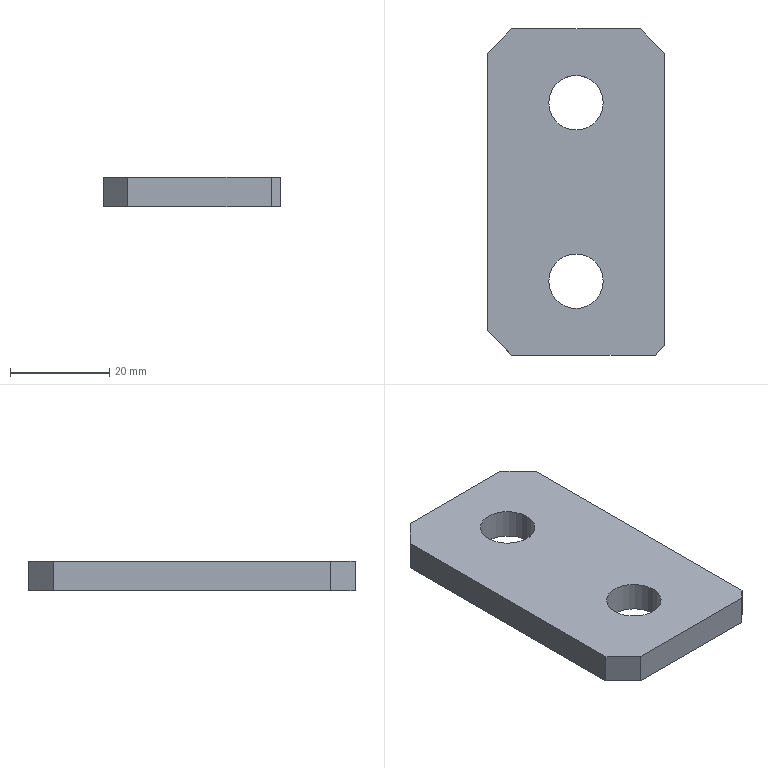Part | STEP file | 1_id134_x_t | 1 solid | 12 faces | box 35.8 x 65.8 x 6 mm | volume 12762 mm3 | plane 10 | cylinder 2 | commonest cylinder face diameters 11 x2
STEP:
#1=CARTESIAN_POINT('',(0.,0.,0.));
#2=DIRECTION('',(0.,0.,1.));
#3=DIRECTION('',(1.,0.,0.));
#4=AXIS2_PLACEMENT_3D('',#1,#2,#3);
#5=CARTESIAN_POINT('',(51.316,210.4,84.11));
#6=VERTEX_POINT('',#5);
#7=CARTESIAN_POINT('',(46.375,205.459,84.11));
#8=VERTEX_POINT('',#7);
#9=CARTESIAN_POINT('',(32.346,191.429,84.11));
#10=DIRECTION('',(-0.7071,-0.7071,0.));
#11=VECTOR('',#10,1.);
#12=LINE('',#9,#11);
#13=CARTESIAN_POINT('',(51.346,210.429,90.11));
#14=DIRECTION('',(0.7071,-0.7071,0.));
#15=DIRECTION('',(0.7071,0.7071,0.));
#16=AXIS2_PLACEMENT_3D('',#13,#14,#15);
#17=PLANE('',#16);
#18=CARTESIAN_POINT('',(-26.87,-6.));
#19=DIRECTION('',(-1.,0.));
#20=VECTOR('',#19,1.);
#21=LINE('',#18,#20);
#22=(GEOMETRIC_REPRESENTATION_CONTEXT(2)PARAMETRIC_REPRESENTATION_CONTEXT()REPRESENTATION_CONTEXT('',''));
#23=DEFINITIONAL_REPRESENTATION('',(#21),#22);
#24=PCURVE('',#17,#23);
#25=CARTESIAN_POINT('',(64.275,159.5,84.11));
#26=DIRECTION('',(0.,0.,-1.));
#27=DIRECTION('',(-1.,0.,0.));
#28=AXIS2_PLACEMENT_3D('',#25,#26,#27);
#29=PLANE('',#28);
#30=CARTESIAN_POINT('',(31.929,31.929));
#31=DIRECTION('',(0.7071,-0.7071));
#32=VECTOR('',#31,1.);
#33=LINE('',#30,#32);
#34=(GEOMETRIC_REPRESENTATION_CONTEXT(2)PARAMETRIC_REPRESENTATION_CONTEXT()REPRESENTATION_CONTEXT('',''));
#35=DEFINITIONAL_REPRESENTATION('',(#33),#34);
#36=PCURVE('',#29,#35);
#37=SURFACE_CURVE('',#12,(#24,#36),.PCURVE_S1.);
#38=EDGE_CURVE('',#6,#8,#37,.T.);
#39=ORIENTED_EDGE('',*,*,#38,.T.);
#40=CARTESIAN_POINT('',(46.375,205.459,90.11));
#41=VERTEX_POINT('',#40);
#42=CARTESIAN_POINT('',(46.375,205.459,90.11));
#43=DIRECTION('',(0.,0.,-1.));
#44=VECTOR('',#43,1.);
#45=LINE('',#42,#44);
#46=CARTESIAN_POINT('',(-7.03,0.));
#47=DIRECTION('',(0.,-1.));
#48=VECTOR('',#47,1.);
#49=LINE('',#46,#48);
#50=(GEOMETRIC_REPRESENTATION_CONTEXT(2)PARAMETRIC_REPRESENTATION_CONTEXT()REPRESENTATION_CONTEXT('',''));
#51=DEFINITIONAL_REPRESENTATION('',(#49),#50);
#52=PCURVE('',#17,#51);
#53=CARTESIAN_POINT('',(46.375,205.5,90.11));
#54=DIRECTION('',(1.,0.,0.));
#55=DIRECTION('',(0.,0.,-1.));
#56=AXIS2_PLACEMENT_3D('',#53,#54,#55);
#57=PLANE('',#56);
#58=CARTESIAN_POINT('',(0.,-0.04142));
#59=DIRECTION('',(1.,0.));
#60=VECTOR('',#59,1.);
#61=LINE('',#58,#60);
#62=(GEOMETRIC_REPRESENTATION_CONTEXT(2)PARAMETRIC_REPRESENTATION_CONTEXT()REPRESENTATION_CONTEXT('',''));
#63=DEFINITIONAL_REPRESENTATION('',(#61),#62);
#64=PCURVE('',#57,#63);
#65=SURFACE_CURVE('',#45,(#52,#64),.PCURVE_S1.);
#66=EDGE_CURVE('',#41,#8,#65,.T.);
#67=ORIENTED_EDGE('',*,*,#66,.F.);
#68=CARTESIAN_POINT('',(51.316,210.4,90.11));
#69=VERTEX_POINT('',#68);
#70=CARTESIAN_POINT('',(32.346,191.429,90.11));
#71=DIRECTION('',(-0.7071,-0.7071,0.));
#72=VECTOR('',#71,1.);
#73=LINE('',#70,#72);
#74=CARTESIAN_POINT('',(-26.87,0.));
#75=DIRECTION('',(-1.,0.));
#76=VECTOR('',#75,1.);
#77=LINE('',#74,#76);
#78=(GEOMETRIC_REPRESENTATION_CONTEXT(2)PARAMETRIC_REPRESENTATION_CONTEXT()REPRESENTATION_CONTEXT('',''));
#79=DEFINITIONAL_REPRESENTATION('',(#77),#78);
#80=PCURVE('',#17,#79);
#81=CARTESIAN_POINT('',(64.275,159.5,90.11));
#82=DIRECTION('',(0.,0.,-1.));
#83=DIRECTION('',(-1.,0.,0.));
#84=AXIS2_PLACEMENT_3D('',#81,#82,#83);
#85=PLANE('',#84);
#86=CARTESIAN_POINT('',(31.929,31.929));
#87=DIRECTION('',(0.7071,-0.7071));
#88=VECTOR('',#87,1.);
#89=LINE('',#86,#88);
#90=(GEOMETRIC_REPRESENTATION_CONTEXT(2)PARAMETRIC_REPRESENTATION_CONTEXT()REPRESENTATION_CONTEXT('',''));
#91=DEFINITIONAL_REPRESENTATION('',(#89),#90);
#92=PCURVE('',#85,#91);
#93=SURFACE_CURVE('',#73,(#80,#92),.PCURVE_S1.);
#94=EDGE_CURVE('',#69,#41,#93,.T.);
#95=ORIENTED_EDGE('',*,*,#94,.F.);
#96=CARTESIAN_POINT('',(51.316,210.4,90.11));
#97=DIRECTION('',(0.,0.,-1.));
#98=VECTOR('',#97,1.);
#99=LINE('',#96,#98);
#100=CARTESIAN_POINT('',(-0.04142,0.));
#101=DIRECTION('',(0.,-1.));
#102=VECTOR('',#101,1.);
#103=LINE('',#100,#102);
#104=(GEOMETRIC_REPRESENTATION_CONTEXT(2)PARAMETRIC_REPRESENTATION_CONTEXT()REPRESENTATION_CONTEXT('',''));
#105=DEFINITIONAL_REPRESENTATION('',(#103),#104);
#106=PCURVE('',#17,#105);
#107=CARTESIAN_POINT('',(77.275,210.4,90.11));
#108=DIRECTION('',(0.,-1.,0.));
#109=DIRECTION('',(0.,0.,-1.));
#110=AXIS2_PLACEMENT_3D('',#107,#108,#109);
#111=PLANE('',#110);
#112=CARTESIAN_POINT('',(0.,-25.959));
#113=DIRECTION('',(1.,0.));
#114=VECTOR('',#113,1.);
#115=LINE('',#112,#114);
#116=(GEOMETRIC_REPRESENTATION_CONTEXT(2)PARAMETRIC_REPRESENTATION_CONTEXT()REPRESENTATION_CONTEXT('',''));
#117=DEFINITIONAL_REPRESENTATION('',(#115),#116);
#118=PCURVE('',#111,#117);
#119=SURFACE_CURVE('',#99,(#106,#118),.PCURVE_S1.);
#120=EDGE_CURVE('',#69,#6,#119,.T.);
#121=ORIENTED_EDGE('',*,*,#120,.T.);
#122=EDGE_LOOP('',(#39,#67,#95,#121));
#123=FACE_BOUND('',#122,.T.);
#124=ADVANCED_FACE('',(#123),#17,.F.);
#125=CARTESIAN_POINT('',(46.375,149.541,84.11));
#126=VERTEX_POINT('',#125);
#127=CARTESIAN_POINT('',(46.375,159.5,84.11));
#128=DIRECTION('',(0.,-1.,0.));
#129=VECTOR('',#128,1.);
#130=LINE('',#127,#129);
#131=CARTESIAN_POINT('',(6.,-46.));
#132=DIRECTION('',(0.,-1.));
#133=VECTOR('',#132,1.);
#134=LINE('',#131,#133);
#135=(GEOMETRIC_REPRESENTATION_CONTEXT(2)PARAMETRIC_REPRESENTATION_CONTEXT()REPRESENTATION_CONTEXT('',''));
#136=DEFINITIONAL_REPRESENTATION('',(#134),#135);
#137=PCURVE('',#57,#136);
#138=CARTESIAN_POINT('',(17.9,0.));
#139=DIRECTION('',(0.,-1.));
#140=VECTOR('',#139,1.);
#141=LINE('',#138,#140);
#142=(GEOMETRIC_REPRESENTATION_CONTEXT(2)PARAMETRIC_REPRESENTATION_CONTEXT()REPRESENTATION_CONTEXT('',''));
#143=DEFINITIONAL_REPRESENTATION('',(#141),#142);
#144=PCURVE('',#29,#143);
#145=SURFACE_CURVE('',#130,(#137,#144),.PCURVE_S1.);
#146=EDGE_CURVE('',#8,#126,#145,.T.);
#147=ORIENTED_EDGE('',*,*,#146,.T.);
#148=CARTESIAN_POINT('',(46.375,149.541,90.11));
#149=VERTEX_POINT('',#148);
#150=CARTESIAN_POINT('',(46.375,149.541,90.11));
#151=DIRECTION('',(0.,0.,-1.));
#152=VECTOR('',#151,1.);
#153=LINE('',#150,#152);
#154=CARTESIAN_POINT('',(0.,-55.959));
#155=DIRECTION('',(1.,0.));
#156=VECTOR('',#155,1.);
#157=LINE('',#154,#156);
#158=(GEOMETRIC_REPRESENTATION_CONTEXT(2)PARAMETRIC_REPRESENTATION_CONTEXT()REPRESENTATION_CONTEXT('',''));
#159=DEFINITIONAL_REPRESENTATION('',(#157),#158);
#160=PCURVE('',#57,#159);
#161=CARTESIAN_POINT('',(46.346,149.571,90.11));
#162=DIRECTION('',(0.7071,0.7071,0.));
#163=DIRECTION('',(-0.7071,0.7071,0.));
#164=AXIS2_PLACEMENT_3D('',#161,#162,#163);
#165=PLANE('',#164);
#166=CARTESIAN_POINT('',(-0.04142,0.));
#167=DIRECTION('',(0.,-1.));
#168=VECTOR('',#167,1.);
#169=LINE('',#166,#168);
#170=(GEOMETRIC_REPRESENTATION_CONTEXT(2)PARAMETRIC_REPRESENTATION_CONTEXT()REPRESENTATION_CONTEXT('',''));
#171=DEFINITIONAL_REPRESENTATION('',(#169),#170);
#172=PCURVE('',#165,#171);
#173=SURFACE_CURVE('',#153,(#160,#172),.PCURVE_S1.);
#174=EDGE_CURVE('',#149,#126,#173,.T.);
#175=ORIENTED_EDGE('',*,*,#174,.F.);
#176=CARTESIAN_POINT('',(46.375,159.5,90.11));
#177=DIRECTION('',(0.,-1.,0.));
#178=VECTOR('',#177,1.);
#179=LINE('',#176,#178);
#180=CARTESIAN_POINT('',(0.,-46.));
#181=DIRECTION('',(0.,-1.));
#182=VECTOR('',#181,1.);
#183=LINE('',#180,#182);
#184=(GEOMETRIC_REPRESENTATION_CONTEXT(2)PARAMETRIC_REPRESENTATION_CONTEXT()REPRESENTATION_CONTEXT('',''));
#185=DEFINITIONAL_REPRESENTATION('',(#183),#184);
#186=PCURVE('',#57,#185);
#187=CARTESIAN_POINT('',(17.9,0.));
#188=DIRECTION('',(0.,-1.));
#189=VECTOR('',#188,1.);
#190=LINE('',#187,#189);
#191=(GEOMETRIC_REPRESENTATION_CONTEXT(2)PARAMETRIC_REPRESENTATION_CONTEXT()REPRESENTATION_CONTEXT('',''));
#192=DEFINITIONAL_REPRESENTATION('',(#190),#191);
#193=PCURVE('',#85,#192);
#194=SURFACE_CURVE('',#179,(#186,#193),.PCURVE_S1.);
#195=EDGE_CURVE('',#41,#149,#194,.T.);
#196=ORIENTED_EDGE('',*,*,#195,.F.);
#197=ORIENTED_EDGE('',*,*,#66,.T.);
#198=EDGE_LOOP('',(#147,#175,#196,#197));
#199=FACE_BOUND('',#198,.T.);
#200=ADVANCED_FACE('',(#199),#57,.F.);
#201=CARTESIAN_POINT('',(51.316,144.6,84.11));
#202=VERTEX_POINT('',#201);
#203=CARTESIAN_POINT('',(50.346,145.571,84.11));
#204=DIRECTION('',(0.7071,-0.7071,0.));
#205=VECTOR('',#204,1.);
#206=LINE('',#203,#205);
#207=CARTESIAN_POINT('',(-5.657,-6.));
#208=DIRECTION('',(-1.,0.));
#209=VECTOR('',#208,1.);
#210=LINE('',#207,#209);
#211=(GEOMETRIC_REPRESENTATION_CONTEXT(2)PARAMETRIC_REPRESENTATION_CONTEXT()REPRESENTATION_CONTEXT('',''));
#212=DEFINITIONAL_REPRESENTATION('',(#210),#211);
#213=PCURVE('',#165,#212);
#214=CARTESIAN_POINT('',(13.929,-13.929));
#215=DIRECTION('',(-0.7071,-0.7071));
#216=VECTOR('',#215,1.);
#217=LINE('',#214,#216);
#218=(GEOMETRIC_REPRESENTATION_CONTEXT(2)PARAMETRIC_REPRESENTATION_CONTEXT()REPRESENTATION_CONTEXT('',''));
#219=DEFINITIONAL_REPRESENTATION('',(#217),#218);
#220=PCURVE('',#29,#219);
#221=SURFACE_CURVE('',#206,(#213,#220),.PCURVE_S1.);
#222=EDGE_CURVE('',#126,#202,#221,.T.);
#223=ORIENTED_EDGE('',*,*,#222,.T.);
#224=CARTESIAN_POINT('',(51.316,144.6,90.11));
#225=VERTEX_POINT('',#224);
#226=CARTESIAN_POINT('',(51.316,144.6,90.11));
#227=DIRECTION('',(0.,0.,-1.));
#228=VECTOR('',#227,1.);
#229=LINE('',#226,#228);
#230=CARTESIAN_POINT('',(-7.03,0.));
#231=DIRECTION('',(0.,-1.));
#232=VECTOR('',#231,1.);
#233=LINE('',#230,#232);
#234=(GEOMETRIC_REPRESENTATION_CONTEXT(2)PARAMETRIC_REPRESENTATION_CONTEXT()REPRESENTATION_CONTEXT('',''));
#235=DEFINITIONAL_REPRESENTATION('',(#233),#234);
#236=PCURVE('',#165,#235);
#237=CARTESIAN_POINT('',(51.275,144.6,90.11));
#238=DIRECTION('',(0.,1.,0.));
#239=DIRECTION('',(0.,0.,1.));
#240=AXIS2_PLACEMENT_3D('',#237,#238,#239);
#241=PLANE('',#240);
#242=CARTESIAN_POINT('',(0.,0.04142));
#243=DIRECTION('',(-1.,0.));
#244=VECTOR('',#243,1.);
#245=LINE('',#242,#244);
#246=(GEOMETRIC_REPRESENTATION_CONTEXT(2)PARAMETRIC_REPRESENTATION_CONTEXT()REPRESENTATION_CONTEXT('',''));
#247=DEFINITIONAL_REPRESENTATION('',(#245),#246);
#248=PCURVE('',#241,#247);
#249=SURFACE_CURVE('',#229,(#236,#248),.PCURVE_S1.);
#250=EDGE_CURVE('',#225,#202,#249,.T.);
#251=ORIENTED_EDGE('',*,*,#250,.F.);
#252=CARTESIAN_POINT('',(50.346,145.571,90.11));
#253=DIRECTION('',(0.7071,-0.7071,0.));
#254=VECTOR('',#253,1.);
#255=LINE('',#252,#254);
#256=CARTESIAN_POINT('',(-5.657,0.));
#257=DIRECTION('',(-1.,0.));
#258=VECTOR('',#257,1.);
#259=LINE('',#256,#258);
#260=(GEOMETRIC_REPRESENTATION_CONTEXT(2)PARAMETRIC_REPRESENTATION_CONTEXT()REPRESENTATION_CONTEXT('',''));
#261=DEFINITIONAL_REPRESENTATION('',(#259),#260);
#262=PCURVE('',#165,#261);
#263=CARTESIAN_POINT('',(13.929,-13.929));
#264=DIRECTION('',(-0.7071,-0.7071));
#265=VECTOR('',#264,1.);
#266=LINE('',#263,#265);
#267=(GEOMETRIC_REPRESENTATION_CONTEXT(2)PARAMETRIC_REPRESENTATION_CONTEXT()REPRESENTATION_CONTEXT('',''));
#268=DEFINITIONAL_REPRESENTATION('',(#266),#267);
#269=PCURVE('',#85,#268);
#270=SURFACE_CURVE('',#255,(#262,#269),.PCURVE_S1.);
#271=EDGE_CURVE('',#149,#225,#270,.T.);
#272=ORIENTED_EDGE('',*,*,#271,.F.);
#273=ORIENTED_EDGE('',*,*,#174,.T.);
#274=EDGE_LOOP('',(#223,#251,#272,#273));
#275=FACE_BOUND('',#274,.T.);
#276=ADVANCED_FACE('',(#275),#165,.F.);
#277=CARTESIAN_POINT('',(58.775,195.5,84.11));
#278=VERTEX_POINT('',#277);
#279=CARTESIAN_POINT('',(64.275,195.5,84.11));
#280=DIRECTION('',(0.,0.,-1.));
#281=DIRECTION('',(-1.,0.,0.));
#282=AXIS2_PLACEMENT_3D('',#279,#280,#281);
#283=CIRCLE('',#282,5.5);
#284=CARTESIAN_POINT('',(64.275,195.5,90.11));
#285=DIRECTION('',(0.,0.,-1.));
#286=DIRECTION('',(-1.,0.,0.));
#287=AXIS2_PLACEMENT_3D('',#284,#285,#286);
#288=CYLINDRICAL_SURFACE('',#287,5.5);
#289=CARTESIAN_POINT('',(0.,6.));
#290=DIRECTION('',(1.,0.));
#291=VECTOR('',#290,1.);
#292=LINE('',#289,#291);
#293=(GEOMETRIC_REPRESENTATION_CONTEXT(2)PARAMETRIC_REPRESENTATION_CONTEXT()REPRESENTATION_CONTEXT('',''));
#294=DEFINITIONAL_REPRESENTATION('',(#292),#293);
#295=PCURVE('',#288,#294);
#296=CARTESIAN_POINT('',(0.,36.));
#297=DIRECTION('',(1.,0.));
#298=AXIS2_PLACEMENT_2D('',#296,#297);
#299=CIRCLE('',#298,5.5);
#300=(GEOMETRIC_REPRESENTATION_CONTEXT(2)PARAMETRIC_REPRESENTATION_CONTEXT()REPRESENTATION_CONTEXT('',''));
#301=DEFINITIONAL_REPRESENTATION('',(#299),#300);
#302=PCURVE('',#29,#301);
#303=SURFACE_CURVE('',#283,(#295,#302),.PCURVE_S1.);
#304=EDGE_CURVE('',#278,#278,#303,.T.);
#305=ORIENTED_EDGE('',*,*,#304,.F.);
#306=CARTESIAN_POINT('',(58.775,195.5,90.11));
#307=VERTEX_POINT('',#306);
#308=CARTESIAN_POINT('',(58.775,195.5,90.11));
#309=CARTESIAN_POINT('',(58.775,195.5,84.11));
#310=B_SPLINE_CURVE_WITH_KNOTS('',1,(#308,#309),.UNSPECIFIED.,.F.,.F.,(2,2),(0.,6.),.PIECEWISE_BEZIER_KNOTS.);
#311=CARTESIAN_POINT('',(0.,0.));
#312=DIRECTION('',(0.,1.));
#313=VECTOR('',#312,1.);
#314=LINE('',#311,#313);
#315=(GEOMETRIC_REPRESENTATION_CONTEXT(2)PARAMETRIC_REPRESENTATION_CONTEXT()REPRESENTATION_CONTEXT('',''));
#316=DEFINITIONAL_REPRESENTATION('',(#314),#315);
#317=PCURVE('',#288,#316);
#318=CARTESIAN_POINT('',(6.283,0.));
#319=DIRECTION('',(0.,1.));
#320=VECTOR('',#319,1.);
#321=LINE('',#318,#320);
#322=(GEOMETRIC_REPRESENTATION_CONTEXT(2)PARAMETRIC_REPRESENTATION_CONTEXT()REPRESENTATION_CONTEXT('',''));
#323=DEFINITIONAL_REPRESENTATION('',(#321),#322);
#324=PCURVE('',#288,#323);
#325=SEAM_CURVE('',#310,(#317,#324),.PCURVE_S1.);
#326=EDGE_CURVE('',#307,#278,#325,.T.);
#327=ORIENTED_EDGE('',*,*,#326,.F.);
#328=CARTESIAN_POINT('',(64.275,195.5,90.11));
#329=DIRECTION('',(0.,0.,-1.));
#330=DIRECTION('',(-1.,0.,0.));
#331=AXIS2_PLACEMENT_3D('',#328,#329,#330);
#332=CIRCLE('',#331,5.5);
#333=CARTESIAN_POINT('',(0.,0.));
#334=DIRECTION('',(1.,0.));
#335=VECTOR('',#334,1.);
#336=LINE('',#333,#335);
#337=(GEOMETRIC_REPRESENTATION_CONTEXT(2)PARAMETRIC_REPRESENTATION_CONTEXT()REPRESENTATION_CONTEXT('',''));
#338=DEFINITIONAL_REPRESENTATION('',(#336),#337);
#339=PCURVE('',#288,#338);
#340=CARTESIAN_POINT('',(0.,36.));
#341=DIRECTION('',(1.,0.));
#342=AXIS2_PLACEMENT_2D('',#340,#341);
#343=CIRCLE('',#342,5.5);
#344=(GEOMETRIC_REPRESENTATION_CONTEXT(2)PARAMETRIC_REPRESENTATION_CONTEXT()REPRESENTATION_CONTEXT('',''));
#345=DEFINITIONAL_REPRESENTATION('',(#343),#344);
#346=PCURVE('',#85,#345);
#347=SURFACE_CURVE('',#332,(#339,#346),.PCURVE_S1.);
#348=EDGE_CURVE('',#307,#307,#347,.T.);
#349=ORIENTED_EDGE('',*,*,#348,.T.);
#350=ORIENTED_EDGE('',*,*,#326,.T.);
#351=EDGE_LOOP('',(#305,#327,#349,#350));
#352=FACE_BOUND('',#351,.F.);
#353=ADVANCED_FACE('',(#352),#288,.F.);
#354=CARTESIAN_POINT('',(58.775,159.5,84.11));
#355=VERTEX_POINT('',#354);
#356=CARTESIAN_POINT('',(64.275,159.5,84.11));
#357=DIRECTION('',(0.,0.,-1.));
#358=DIRECTION('',(-1.,0.,0.));
#359=AXIS2_PLACEMENT_3D('',#356,#357,#358);
#360=CIRCLE('',#359,5.5);
#361=CARTESIAN_POINT('',(64.275,159.5,90.11));
#362=DIRECTION('',(0.,0.,-1.));
#363=DIRECTION('',(-1.,0.,0.));
#364=AXIS2_PLACEMENT_3D('',#361,#362,#363);
#365=CYLINDRICAL_SURFACE('',#364,5.5);
#366=CARTESIAN_POINT('',(0.,6.));
#367=DIRECTION('',(1.,0.));
#368=VECTOR('',#367,1.);
#369=LINE('',#366,#368);
#370=(GEOMETRIC_REPRESENTATION_CONTEXT(2)PARAMETRIC_REPRESENTATION_CONTEXT()REPRESENTATION_CONTEXT('',''));
#371=DEFINITIONAL_REPRESENTATION('',(#369),#370);
#372=PCURVE('',#365,#371);
#373=CARTESIAN_POINT('',(0.,0.));
#374=DIRECTION('',(1.,0.));
#375=AXIS2_PLACEMENT_2D('',#373,#374);
#376=CIRCLE('',#375,5.5);
#377=(GEOMETRIC_REPRESENTATION_CONTEXT(2)PARAMETRIC_REPRESENTATION_CONTEXT()REPRESENTATION_CONTEXT('',''));
#378=DEFINITIONAL_REPRESENTATION('',(#376),#377);
#379=PCURVE('',#29,#378);
#380=SURFACE_CURVE('',#360,(#372,#379),.PCURVE_S1.);
#381=EDGE_CURVE('',#355,#355,#380,.T.);
#382=ORIENTED_EDGE('',*,*,#381,.F.);
#383=CARTESIAN_POINT('',(58.775,159.5,90.11));
#384=VERTEX_POINT('',#383);
#385=CARTESIAN_POINT('',(58.775,159.5,90.11));
#386=CARTESIAN_POINT('',(58.775,159.5,84.11));
#387=B_SPLINE_CURVE_WITH_KNOTS('',1,(#385,#386),.UNSPECIFIED.,.F.,.F.,(2,2),(0.,6.),.PIECEWISE_BEZIER_KNOTS.);
#388=CARTESIAN_POINT('',(0.,0.));
#389=DIRECTION('',(0.,1.));
#390=VECTOR('',#389,1.);
#391=LINE('',#388,#390);
#392=(GEOMETRIC_REPRESENTATION_CONTEXT(2)PARAMETRIC_REPRESENTATION_CONTEXT()REPRESENTATION_CONTEXT('',''));
#393=DEFINITIONAL_REPRESENTATION('',(#391),#392);
#394=PCURVE('',#365,#393);
#395=CARTESIAN_POINT('',(6.283,0.));
#396=DIRECTION('',(0.,1.));
#397=VECTOR('',#396,1.);
#398=LINE('',#395,#397);
#399=(GEOMETRIC_REPRESENTATION_CONTEXT(2)PARAMETRIC_REPRESENTATION_CONTEXT()REPRESENTATION_CONTEXT('',''));
#400=DEFINITIONAL_REPRESENTATION('',(#398),#399);
#401=PCURVE('',#365,#400);
#402=SEAM_CURVE('',#387,(#394,#401),.PCURVE_S1.);
#403=EDGE_CURVE('',#384,#355,#402,.T.);
#404=ORIENTED_EDGE('',*,*,#403,.F.);
#405=CARTESIAN_POINT('',(64.275,159.5,90.11));
#406=DIRECTION('',(0.,0.,-1.));
#407=DIRECTION('',(-1.,0.,0.));
#408=AXIS2_PLACEMENT_3D('',#405,#406,#407);
#409=CIRCLE('',#408,5.5);
#410=CARTESIAN_POINT('',(0.,0.));
#411=DIRECTION('',(1.,0.));
#412=VECTOR('',#411,1.);
#413=LINE('',#410,#412);
#414=(GEOMETRIC_REPRESENTATION_CONTEXT(2)PARAMETRIC_REPRESENTATION_CONTEXT()REPRESENTATION_CONTEXT('',''));
#415=DEFINITIONAL_REPRESENTATION('',(#413),#414);
#416=PCURVE('',#365,#415);
#417=CARTESIAN_POINT('',(0.,0.));
#418=DIRECTION('',(1.,0.));
#419=AXIS2_PLACEMENT_2D('',#417,#418);
#420=CIRCLE('',#419,5.5);
#421=(GEOMETRIC_REPRESENTATION_CONTEXT(2)PARAMETRIC_REPRESENTATION_CONTEXT()REPRESENTATION_CONTEXT('',''));
#422=DEFINITIONAL_REPRESENTATION('',(#420),#421);
#423=PCURVE('',#85,#422);
#424=SURFACE_CURVE('',#409,(#416,#423),.PCURVE_S1.);
#425=EDGE_CURVE('',#384,#384,#424,.T.);
#426=ORIENTED_EDGE('',*,*,#425,.T.);
#427=ORIENTED_EDGE('',*,*,#403,.T.);
#428=EDGE_LOOP('',(#382,#404,#426,#427));
#429=FACE_BOUND('',#428,.F.);
#430=ADVANCED_FACE('',(#429),#365,.F.);
#431=ORIENTED_EDGE('',*,*,#425,.T.);
#432=EDGE_LOOP('',(#431));
#433=FACE_BOUND('',#432,.T.);
#434=ORIENTED_EDGE('',*,*,#348,.T.);
#435=EDGE_LOOP('',(#434));
#436=FACE_BOUND('',#435,.T.);
#437=CARTESIAN_POINT('',(82.175,146.541,90.11));
#438=VERTEX_POINT('',#437);
#439=CARTESIAN_POINT('',(80.234,144.6,90.11));
#440=VERTEX_POINT('',#439);
#441=CARTESIAN_POINT('',(79.704,144.071,90.11));
#442=DIRECTION('',(-0.7071,-0.7071,0.));
#443=VECTOR('',#442,1.);
#444=LINE('',#441,#443);
#445=CARTESIAN_POINT('',(-15.429,-15.429));
#446=DIRECTION('',(0.7071,-0.7071));
#447=VECTOR('',#446,1.);
#448=LINE('',#445,#447);
#449=(GEOMETRIC_REPRESENTATION_CONTEXT(2)PARAMETRIC_REPRESENTATION_CONTEXT()REPRESENTATION_CONTEXT('',''));
#450=DEFINITIONAL_REPRESENTATION('',(#448),#449);
#451=PCURVE('',#85,#450);
#452=CARTESIAN_POINT('',(80.234,144.6,-90.11));
#453=DIRECTION('',(0.7071,-0.7071,0.));
#454=DIRECTION('',(0.7071,0.7071,0.));
#455=AXIS2_PLACEMENT_3D('',#452,#453,#454);
#456=PLANE('',#455);
#457=CARTESIAN_POINT('',(-0.7485,180.22));
#458=DIRECTION('',(-1.,0.));
#459=VECTOR('',#458,1.);
#460=LINE('',#457,#459);
#461=(GEOMETRIC_REPRESENTATION_CONTEXT(2)PARAMETRIC_REPRESENTATION_CONTEXT()REPRESENTATION_CONTEXT('',''));
#462=DEFINITIONAL_REPRESENTATION('',(#460),#461);
#463=PCURVE('',#456,#462);
#464=SURFACE_CURVE('',#444,(#451,#463),.PCURVE_S1.);
#465=EDGE_CURVE('',#438,#440,#464,.T.);
#466=ORIENTED_EDGE('',*,*,#465,.F.);
#467=CARTESIAN_POINT('',(82.175,205.459,90.11));
#468=VERTEX_POINT('',#467);
#469=CARTESIAN_POINT('',(82.175,159.5,90.11));
#470=DIRECTION('',(0.,1.,0.));
#471=VECTOR('',#470,1.);
#472=LINE('',#469,#471);
#473=CARTESIAN_POINT('',(-17.9,0.));
#474=DIRECTION('',(0.,1.));
#475=VECTOR('',#474,1.);
#476=LINE('',#473,#475);
#477=(GEOMETRIC_REPRESENTATION_CONTEXT(2)PARAMETRIC_REPRESENTATION_CONTEXT()REPRESENTATION_CONTEXT('',''));
#478=DEFINITIONAL_REPRESENTATION('',(#476),#477);
#479=PCURVE('',#85,#478);
#480=CARTESIAN_POINT('',(82.175,149.5,90.11));
#481=DIRECTION('',(-1.,0.,0.));
#482=DIRECTION('',(0.,0.,1.));
#483=AXIS2_PLACEMENT_3D('',#480,#481,#482);
#484=PLANE('',#483);
#485=CARTESIAN_POINT('',(0.,10.));
#486=DIRECTION('',(0.,1.));
#487=VECTOR('',#486,1.);
#488=LINE('',#485,#487);
#489=(GEOMETRIC_REPRESENTATION_CONTEXT(2)PARAMETRIC_REPRESENTATION_CONTEXT()REPRESENTATION_CONTEXT('',''));
#490=DEFINITIONAL_REPRESENTATION('',(#488),#489);
#491=PCURVE('',#484,#490);
#492=SURFACE_CURVE('',#472,(#479,#491),.PCURVE_S1.);
#493=EDGE_CURVE('',#438,#468,#492,.T.);
#494=ORIENTED_EDGE('',*,*,#493,.T.);
#495=CARTESIAN_POINT('',(77.234,210.4,90.11));
#496=VERTEX_POINT('',#495);
#497=CARTESIAN_POINT('',(96.204,191.429,90.11));
#498=DIRECTION('',(0.7071,-0.7071,0.));
#499=VECTOR('',#498,1.);
#500=LINE('',#497,#499);
#501=CARTESIAN_POINT('',(-31.929,31.929));
#502=DIRECTION('',(-0.7071,-0.7071));
#503=VECTOR('',#502,1.);
#504=LINE('',#501,#503);
#505=(GEOMETRIC_REPRESENTATION_CONTEXT(2)PARAMETRIC_REPRESENTATION_CONTEXT()REPRESENTATION_CONTEXT('',''));
#506=DEFINITIONAL_REPRESENTATION('',(#504),#505);
#507=PCURVE('',#85,#506);
#508=CARTESIAN_POINT('',(82.175,205.459,-90.11));
#509=DIRECTION('',(0.7071,0.7071,0.));
#510=DIRECTION('',(-0.7071,0.7071,0.));
#511=AXIS2_PLACEMENT_3D('',#508,#509,#510);
#512=PLANE('',#511);
#513=CARTESIAN_POINT('',(-19.84,180.22));
#514=DIRECTION('',(-1.,0.));
#515=VECTOR('',#514,1.);
#516=LINE('',#513,#515);
#517=(GEOMETRIC_REPRESENTATION_CONTEXT(2)PARAMETRIC_REPRESENTATION_CONTEXT()REPRESENTATION_CONTEXT('',''));
#518=DEFINITIONAL_REPRESENTATION('',(#516),#517);
#519=PCURVE('',#512,#518);
#520=SURFACE_CURVE('',#500,(#507,#519),.PCURVE_S1.);
#521=EDGE_CURVE('',#496,#468,#520,.T.);
#522=ORIENTED_EDGE('',*,*,#521,.F.);
#523=CARTESIAN_POINT('',(64.275,210.4,90.11));
#524=DIRECTION('',(-1.,0.,0.));
#525=VECTOR('',#524,1.);
#526=LINE('',#523,#525);
#527=CARTESIAN_POINT('',(0.,50.9));
#528=DIRECTION('',(1.,0.));
#529=VECTOR('',#528,1.);
#530=LINE('',#527,#529);
#531=(GEOMETRIC_REPRESENTATION_CONTEXT(2)PARAMETRIC_REPRESENTATION_CONTEXT()REPRESENTATION_CONTEXT('',''));
#532=DEFINITIONAL_REPRESENTATION('',(#530),#531);
#533=PCURVE('',#85,#532);
#534=CARTESIAN_POINT('',(0.,-13.));
#535=DIRECTION('',(0.,-1.));
#536=VECTOR('',#535,1.);
#537=LINE('',#534,#536);
#538=(GEOMETRIC_REPRESENTATION_CONTEXT(2)PARAMETRIC_REPRESENTATION_CONTEXT()REPRESENTATION_CONTEXT('',''));
#539=DEFINITIONAL_REPRESENTATION('',(#537),#538);
#540=PCURVE('',#111,#539);
#541=SURFACE_CURVE('',#526,(#533,#540),.PCURVE_S1.);
#542=EDGE_CURVE('',#496,#69,#541,.T.);
#543=ORIENTED_EDGE('',*,*,#542,.T.);
#544=ORIENTED_EDGE('',*,*,#94,.T.);
#545=ORIENTED_EDGE('',*,*,#195,.T.);
#546=ORIENTED_EDGE('',*,*,#271,.T.);
#547=CARTESIAN_POINT('',(64.275,144.6,90.11));
#548=DIRECTION('',(1.,0.,0.));
#549=VECTOR('',#548,1.);
#550=LINE('',#547,#549);
#551=CARTESIAN_POINT('',(0.,-14.9));
#552=DIRECTION('',(-1.,0.));
#553=VECTOR('',#552,1.);
#554=LINE('',#551,#553);
#555=(GEOMETRIC_REPRESENTATION_CONTEXT(2)PARAMETRIC_REPRESENTATION_CONTEXT()REPRESENTATION_CONTEXT('',''));
#556=DEFINITIONAL_REPRESENTATION('',(#554),#555);
#557=PCURVE('',#85,#556);
#558=CARTESIAN_POINT('',(0.,13.));
#559=DIRECTION('',(0.,1.));
#560=VECTOR('',#559,1.);
#561=LINE('',#558,#560);
#562=(GEOMETRIC_REPRESENTATION_CONTEXT(2)PARAMETRIC_REPRESENTATION_CONTEXT()REPRESENTATION_CONTEXT('',''));
#563=DEFINITIONAL_REPRESENTATION('',(#561),#562);
#564=PCURVE('',#241,#563);
#565=SURFACE_CURVE('',#550,(#557,#564),.PCURVE_S1.);
#566=EDGE_CURVE('',#225,#440,#565,.T.);
#567=ORIENTED_EDGE('',*,*,#566,.T.);
#568=EDGE_LOOP('',(#466,#494,#522,#543,#544,#545,#546,#567));
#569=FACE_BOUND('',#568,.T.);
#570=ADVANCED_FACE('',(#433,#436,#569),#85,.F.);
#571=ORIENTED_EDGE('',*,*,#381,.F.);
#572=EDGE_LOOP('',(#571));
#573=FACE_BOUND('',#572,.T.);
#574=ORIENTED_EDGE('',*,*,#304,.F.);
#575=EDGE_LOOP('',(#574));
#576=FACE_BOUND('',#575,.T.);
#577=CARTESIAN_POINT('',(82.175,146.541,84.11));
#578=VERTEX_POINT('',#577);
#579=CARTESIAN_POINT('',(82.175,205.459,84.11));
#580=VERTEX_POINT('',#579);
#581=CARTESIAN_POINT('',(82.175,159.5,84.11));
#582=DIRECTION('',(0.,1.,0.));
#583=VECTOR('',#582,1.);
#584=LINE('',#581,#583);
#585=CARTESIAN_POINT('',(-17.9,0.));
#586=DIRECTION('',(0.,1.));
#587=VECTOR('',#586,1.);
#588=LINE('',#585,#587);
#589=(GEOMETRIC_REPRESENTATION_CONTEXT(2)PARAMETRIC_REPRESENTATION_CONTEXT()REPRESENTATION_CONTEXT('',''));
#590=DEFINITIONAL_REPRESENTATION('',(#588),#589);
#591=PCURVE('',#29,#590);
#592=CARTESIAN_POINT('',(-6.,10.));
#593=DIRECTION('',(0.,1.));
#594=VECTOR('',#593,1.);
#595=LINE('',#592,#594);
#596=(GEOMETRIC_REPRESENTATION_CONTEXT(2)PARAMETRIC_REPRESENTATION_CONTEXT()REPRESENTATION_CONTEXT('',''));
#597=DEFINITIONAL_REPRESENTATION('',(#595),#596);
#598=PCURVE('',#484,#597);
#599=SURFACE_CURVE('',#584,(#591,#598),.PCURVE_S1.);
#600=EDGE_CURVE('',#578,#580,#599,.T.);
#601=ORIENTED_EDGE('',*,*,#600,.F.);
#602=CARTESIAN_POINT('',(80.234,144.6,84.11));
#603=VERTEX_POINT('',#602);
#604=CARTESIAN_POINT('',(79.704,144.071,84.11));
#605=DIRECTION('',(-0.7071,-0.7071,0.));
#606=VECTOR('',#605,1.);
#607=LINE('',#604,#606);
#608=CARTESIAN_POINT('',(-15.429,-15.429));
#609=DIRECTION('',(0.7071,-0.7071));
#610=VECTOR('',#609,1.);
#611=LINE('',#608,#610);
#612=(GEOMETRIC_REPRESENTATION_CONTEXT(2)PARAMETRIC_REPRESENTATION_CONTEXT()REPRESENTATION_CONTEXT('',''));
#613=DEFINITIONAL_REPRESENTATION('',(#611),#612);
#614=PCURVE('',#29,#613);
#615=CARTESIAN_POINT('',(-0.7485,174.22));
#616=DIRECTION('',(-1.,0.));
#617=VECTOR('',#616,1.);
#618=LINE('',#615,#617);
#619=(GEOMETRIC_REPRESENTATION_CONTEXT(2)PARAMETRIC_REPRESENTATION_CONTEXT()REPRESENTATION_CONTEXT('',''));
#620=DEFINITIONAL_REPRESENTATION('',(#618),#619);
#621=PCURVE('',#456,#620);
#622=SURFACE_CURVE('',#607,(#614,#621),.PCURVE_S1.);
#623=EDGE_CURVE('',#578,#603,#622,.T.);
#624=ORIENTED_EDGE('',*,*,#623,.T.);
#625=CARTESIAN_POINT('',(64.275,144.6,84.11));
#626=DIRECTION('',(1.,0.,0.));
#627=VECTOR('',#626,1.);
#628=LINE('',#625,#627);
#629=CARTESIAN_POINT('',(0.,-14.9));
#630=DIRECTION('',(-1.,0.));
#631=VECTOR('',#630,1.);
#632=LINE('',#629,#631);
#633=(GEOMETRIC_REPRESENTATION_CONTEXT(2)PARAMETRIC_REPRESENTATION_CONTEXT()REPRESENTATION_CONTEXT('',''));
#634=DEFINITIONAL_REPRESENTATION('',(#632),#633);
#635=PCURVE('',#29,#634);
#636=CARTESIAN_POINT('',(-6.,13.));
#637=DIRECTION('',(0.,1.));
#638=VECTOR('',#637,1.);
#639=LINE('',#636,#638);
#640=(GEOMETRIC_REPRESENTATION_CONTEXT(2)PARAMETRIC_REPRESENTATION_CONTEXT()REPRESENTATION_CONTEXT('',''));
#641=DEFINITIONAL_REPRESENTATION('',(#639),#640);
#642=PCURVE('',#241,#641);
#643=SURFACE_CURVE('',#628,(#635,#642),.PCURVE_S1.);
#644=EDGE_CURVE('',#202,#603,#643,.T.);
#645=ORIENTED_EDGE('',*,*,#644,.F.);
#646=ORIENTED_EDGE('',*,*,#222,.F.);
#647=ORIENTED_EDGE('',*,*,#146,.F.);
#648=ORIENTED_EDGE('',*,*,#38,.F.);
#649=CARTESIAN_POINT('',(77.234,210.4,84.11));
#650=VERTEX_POINT('',#649);
#651=CARTESIAN_POINT('',(64.275,210.4,84.11));
#652=DIRECTION('',(-1.,0.,0.));
#653=VECTOR('',#652,1.);
#654=LINE('',#651,#653);
#655=CARTESIAN_POINT('',(0.,50.9));
#656=DIRECTION('',(1.,0.));
#657=VECTOR('',#656,1.);
#658=LINE('',#655,#657);
#659=(GEOMETRIC_REPRESENTATION_CONTEXT(2)PARAMETRIC_REPRESENTATION_CONTEXT()REPRESENTATION_CONTEXT('',''));
#660=DEFINITIONAL_REPRESENTATION('',(#658),#659);
#661=PCURVE('',#29,#660);
#662=CARTESIAN_POINT('',(6.,-13.));
#663=DIRECTION('',(0.,-1.));
#664=VECTOR('',#663,1.);
#665=LINE('',#662,#664);
#666=(GEOMETRIC_REPRESENTATION_CONTEXT(2)PARAMETRIC_REPRESENTATION_CONTEXT()REPRESENTATION_CONTEXT('',''));
#667=DEFINITIONAL_REPRESENTATION('',(#665),#666);
#668=PCURVE('',#111,#667);
#669=SURFACE_CURVE('',#654,(#661,#668),.PCURVE_S1.);
#670=EDGE_CURVE('',#650,#6,#669,.T.);
#671=ORIENTED_EDGE('',*,*,#670,.F.);
#672=CARTESIAN_POINT('',(96.204,191.429,84.11));
#673=DIRECTION('',(0.7071,-0.7071,0.));
#674=VECTOR('',#673,1.);
#675=LINE('',#672,#674);
#676=CARTESIAN_POINT('',(-31.929,31.929));
#677=DIRECTION('',(-0.7071,-0.7071));
#678=VECTOR('',#677,1.);
#679=LINE('',#676,#678);
#680=(GEOMETRIC_REPRESENTATION_CONTEXT(2)PARAMETRIC_REPRESENTATION_CONTEXT()REPRESENTATION_CONTEXT('',''));
#681=DEFINITIONAL_REPRESENTATION('',(#679),#680);
#682=PCURVE('',#29,#681);
#683=CARTESIAN_POINT('',(-19.84,174.22));
#684=DIRECTION('',(-1.,0.));
#685=VECTOR('',#684,1.);
#686=LINE('',#683,#685);
#687=(GEOMETRIC_REPRESENTATION_CONTEXT(2)PARAMETRIC_REPRESENTATION_CONTEXT()REPRESENTATION_CONTEXT('',''));
#688=DEFINITIONAL_REPRESENTATION('',(#686),#687);
#689=PCURVE('',#512,#688);
#690=SURFACE_CURVE('',#675,(#682,#689),.PCURVE_S1.);
#691=EDGE_CURVE('',#650,#580,#690,.T.);
#692=ORIENTED_EDGE('',*,*,#691,.T.);
#693=EDGE_LOOP('',(#601,#624,#645,#646,#647,#648,#671,#692));
#694=FACE_BOUND('',#693,.T.);
#695=ADVANCED_FACE('',(#573,#576,#694),#29,.T.);
#696=CARTESIAN_POINT('',(77.234,210.4,-90.11));
#697=DIRECTION('',(0.,0.,1.));
#698=VECTOR('',#697,1.);
#699=LINE('',#696,#698);
#700=CARTESIAN_POINT('',(180.22,-0.04142));
#701=DIRECTION('',(-1.,0.));
#702=VECTOR('',#701,1.);
#703=LINE('',#700,#702);
#704=(GEOMETRIC_REPRESENTATION_CONTEXT(2)PARAMETRIC_REPRESENTATION_CONTEXT()REPRESENTATION_CONTEXT('',''));
#705=DEFINITIONAL_REPRESENTATION('',(#703),#704);
#706=PCURVE('',#111,#705);
#707=CARTESIAN_POINT('',(6.988,0.));
#708=DIRECTION('',(0.,1.));
#709=VECTOR('',#708,1.);
#710=LINE('',#707,#709);
#711=(GEOMETRIC_REPRESENTATION_CONTEXT(2)PARAMETRIC_REPRESENTATION_CONTEXT()REPRESENTATION_CONTEXT('',''));
#712=DEFINITIONAL_REPRESENTATION('',(#710),#711);
#713=PCURVE('',#512,#712);
#714=SURFACE_CURVE('',#699,(#706,#713),.PCURVE_S1.);
#715=EDGE_CURVE('',#650,#496,#714,.T.);
#716=ORIENTED_EDGE('',*,*,#715,.F.);
#717=ORIENTED_EDGE('',*,*,#670,.T.);
#718=ORIENTED_EDGE('',*,*,#120,.F.);
#719=ORIENTED_EDGE('',*,*,#542,.F.);
#720=EDGE_LOOP('',(#716,#717,#718,#719));
#721=FACE_BOUND('',#720,.T.);
#722=ADVANCED_FACE('',(#721),#111,.F.);
#723=CARTESIAN_POINT('',(82.175,146.541,-90.11));
#724=DIRECTION('',(0.,0.,1.));
#725=VECTOR('',#724,1.);
#726=LINE('',#723,#725);
#727=CARTESIAN_POINT('',(-180.22,-2.959));
#728=DIRECTION('',(1.,0.));
#729=VECTOR('',#728,1.);
#730=LINE('',#727,#729);
#731=(GEOMETRIC_REPRESENTATION_CONTEXT(2)PARAMETRIC_REPRESENTATION_CONTEXT()REPRESENTATION_CONTEXT('',''));
#732=DEFINITIONAL_REPRESENTATION('',(#730),#731);
#733=PCURVE('',#484,#732);
#734=CARTESIAN_POINT('',(2.746,0.));
#735=DIRECTION('',(0.,1.));
#736=VECTOR('',#735,1.);
#737=LINE('',#734,#736);
#738=(GEOMETRIC_REPRESENTATION_CONTEXT(2)PARAMETRIC_REPRESENTATION_CONTEXT()REPRESENTATION_CONTEXT('',''));
#739=DEFINITIONAL_REPRESENTATION('',(#737),#738);
#740=PCURVE('',#456,#739);
#741=SURFACE_CURVE('',#726,(#733,#740),.PCURVE_S1.);
#742=EDGE_CURVE('',#578,#438,#741,.T.);
#743=ORIENTED_EDGE('',*,*,#742,.F.);
#744=ORIENTED_EDGE('',*,*,#600,.T.);
#745=CARTESIAN_POINT('',(82.175,205.459,-90.11));
#746=DIRECTION('',(0.,0.,1.));
#747=VECTOR('',#746,1.);
#748=LINE('',#745,#747);
#749=CARTESIAN_POINT('',(-180.22,55.959));
#750=DIRECTION('',(1.,0.));
#751=VECTOR('',#750,1.);
#752=LINE('',#749,#751);
#753=(GEOMETRIC_REPRESENTATION_CONTEXT(2)PARAMETRIC_REPRESENTATION_CONTEXT()REPRESENTATION_CONTEXT('',''));
#754=DEFINITIONAL_REPRESENTATION('',(#752),#753);
#755=PCURVE('',#484,#754);
#756=CARTESIAN_POINT('',(0.,0.));
#757=DIRECTION('',(0.,1.));
#758=VECTOR('',#757,1.);
#759=LINE('',#756,#758);
#760=(GEOMETRIC_REPRESENTATION_CONTEXT(2)PARAMETRIC_REPRESENTATION_CONTEXT()REPRESENTATION_CONTEXT('',''));
#761=DEFINITIONAL_REPRESENTATION('',(#759),#760);
#762=PCURVE('',#512,#761);
#763=SURFACE_CURVE('',#748,(#755,#762),.PCURVE_S1.);
#764=EDGE_CURVE('',#580,#468,#763,.T.);
#765=ORIENTED_EDGE('',*,*,#764,.T.);
#766=ORIENTED_EDGE('',*,*,#493,.F.);
#767=EDGE_LOOP('',(#743,#744,#765,#766));
#768=FACE_BOUND('',#767,.T.);
#769=ADVANCED_FACE('',(#768),#484,.F.);
#770=ORIENTED_EDGE('',*,*,#644,.T.);
#771=CARTESIAN_POINT('',(80.234,144.6,-90.11));
#772=DIRECTION('',(0.,0.,1.));
#773=VECTOR('',#772,1.);
#774=LINE('',#771,#773);
#775=CARTESIAN_POINT('',(-180.22,28.959));
#776=DIRECTION('',(1.,0.));
#777=VECTOR('',#776,1.);
#778=LINE('',#775,#777);
#779=(GEOMETRIC_REPRESENTATION_CONTEXT(2)PARAMETRIC_REPRESENTATION_CONTEXT()REPRESENTATION_CONTEXT('',''));
#780=DEFINITIONAL_REPRESENTATION('',(#778),#779);
#781=PCURVE('',#241,#780);
#782=CARTESIAN_POINT('',(0.,0.));
#783=DIRECTION('',(0.,1.));
#784=VECTOR('',#783,1.);
#785=LINE('',#782,#784);
#786=(GEOMETRIC_REPRESENTATION_CONTEXT(2)PARAMETRIC_REPRESENTATION_CONTEXT()REPRESENTATION_CONTEXT('',''));
#787=DEFINITIONAL_REPRESENTATION('',(#785),#786);
#788=PCURVE('',#456,#787);
#789=SURFACE_CURVE('',#774,(#781,#788),.PCURVE_S1.);
#790=EDGE_CURVE('',#603,#440,#789,.T.);
#791=ORIENTED_EDGE('',*,*,#790,.T.);
#792=ORIENTED_EDGE('',*,*,#566,.F.);
#793=ORIENTED_EDGE('',*,*,#250,.T.);
#794=EDGE_LOOP('',(#770,#791,#792,#793));
#795=FACE_BOUND('',#794,.T.);
#796=ADVANCED_FACE('',(#795),#241,.F.);
#797=ORIENTED_EDGE('',*,*,#715,.T.);
#798=ORIENTED_EDGE('',*,*,#521,.T.);
#799=ORIENTED_EDGE('',*,*,#764,.F.);
#800=ORIENTED_EDGE('',*,*,#691,.F.);
#801=EDGE_LOOP('',(#797,#798,#799,#800));
#802=FACE_BOUND('',#801,.T.);
#803=ADVANCED_FACE('',(#802),#512,.T.);
#804=ORIENTED_EDGE('',*,*,#742,.T.);
#805=ORIENTED_EDGE('',*,*,#465,.T.);
#806=ORIENTED_EDGE('',*,*,#790,.F.);
#807=ORIENTED_EDGE('',*,*,#623,.F.);
#808=EDGE_LOOP('',(#804,#805,#806,#807));
#809=FACE_BOUND('',#808,.T.);
#810=ADVANCED_FACE('',(#809),#456,.T.);
#811=CLOSED_SHELL('',(#124,#200,#276,#353,#430,#570,#695,#722,#769,#796,#803,#810));
#812=MANIFOLD_SOLID_BREP('',#811);
#813=(LENGTH_UNIT()NAMED_UNIT(*)SI_UNIT(.MILLI.,.METRE.));
#814=UNCERTAINTY_MEASURE_WITH_UNIT(LENGTH_MEASURE(0.000002),#813,'','');
#815=(NAMED_UNIT(*)PLANE_ANGLE_UNIT()SI_UNIT($,.RADIAN.));
#816=(NAMED_UNIT(*)SI_UNIT($,.STERADIAN.)SOLID_ANGLE_UNIT());
#817=(GEOMETRIC_REPRESENTATION_CONTEXT(3)GLOBAL_UNCERTAINTY_ASSIGNED_CONTEXT((#814))GLOBAL_UNIT_ASSIGNED_CONTEXT((#813,#815,#816))REPRESENTATION_CONTEXT('',''));
#818=ADVANCED_BREP_SHAPE_REPRESENTATION('',(#4,#812),#817);